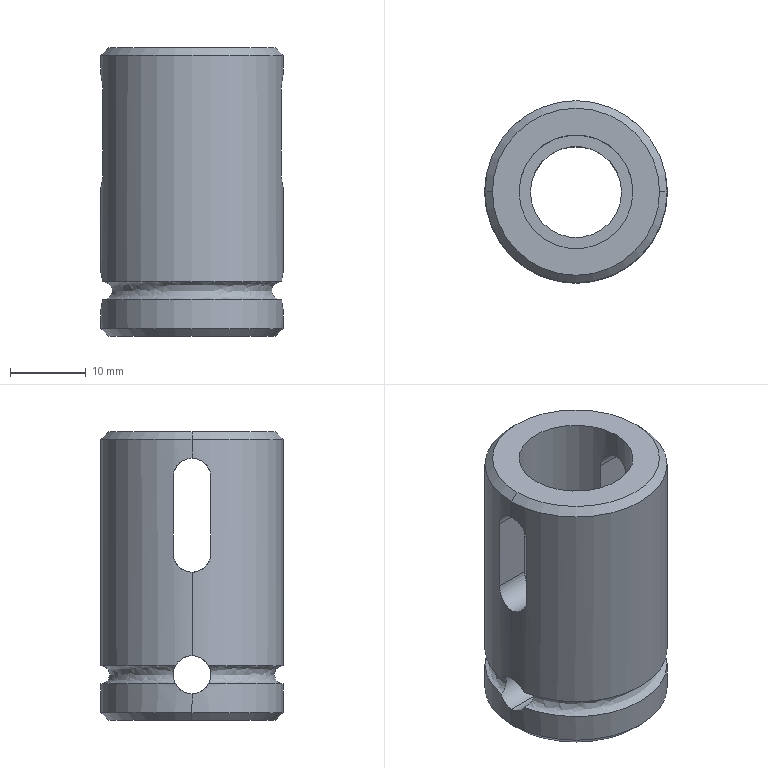Part | STEP file | fBY02F02M-00-17A | 1 solid | 31 faces | box 24 x 24 x 38 mm | volume 10216 mm3 | cylinder 18 | plane 7 | cone 4 | spline 2 | commonest cylinder face diameters 5 x10 24 x4 12 x2 15 x2